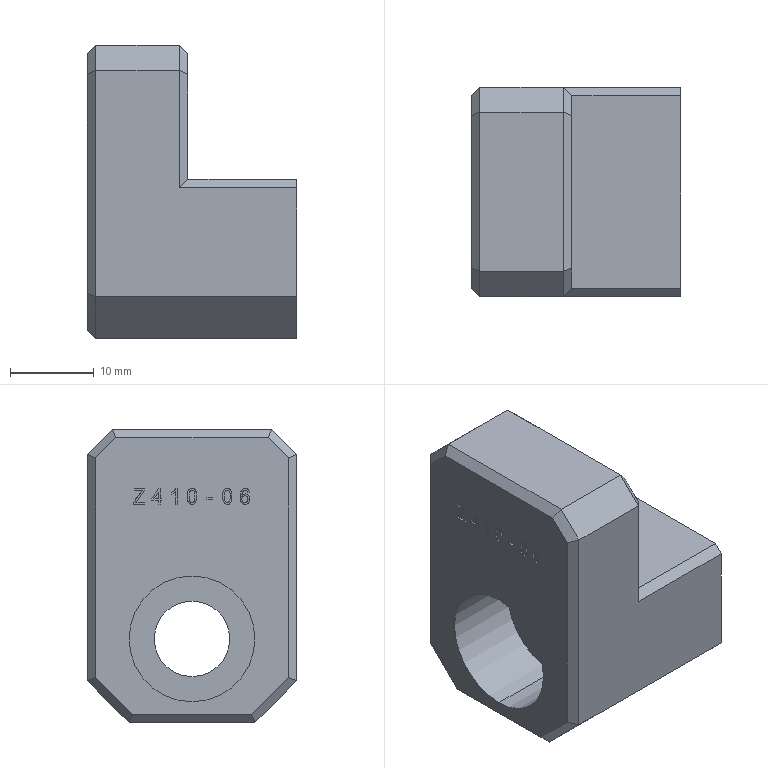Part | Creo | 1 solid | 150 faces | box 25 x 25 x 35 mm | volume 13239 mm3 | other 77 | plane 68 | cylinder 5 | commonest cylinder face diameters 9 x2 15 x2 25.767 x1